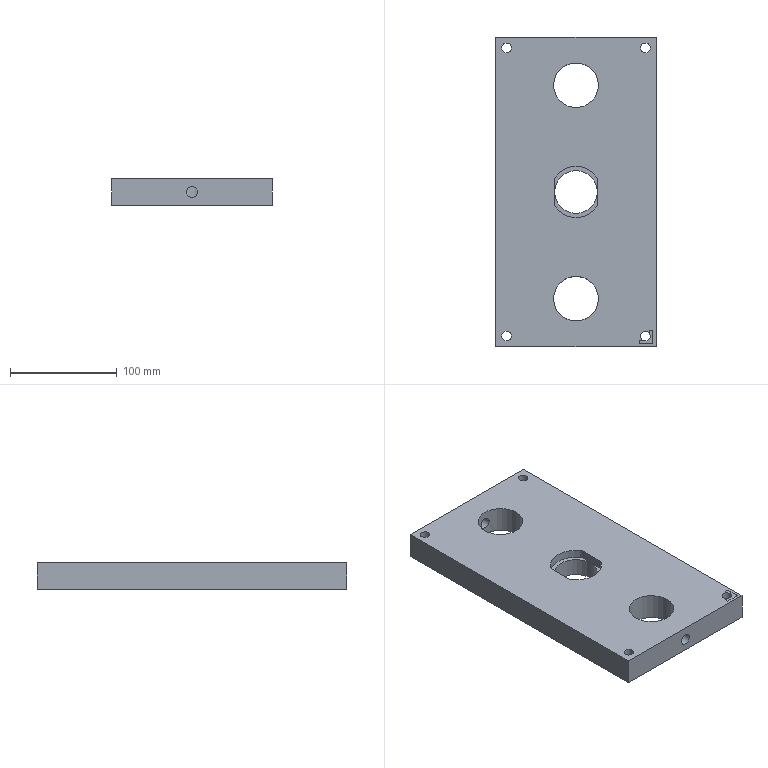Part | STEP file | DZDB_id254_x_t | 1 solid | 63 faces | box 150 x 290 x 25 mm | volume 967966 mm3 | cylinder 37 | plane 20 | cone 6 | commonest cylinder face diameters 6 x12 5 x6 9 x4 10 x4 14 x4 10.5 x2